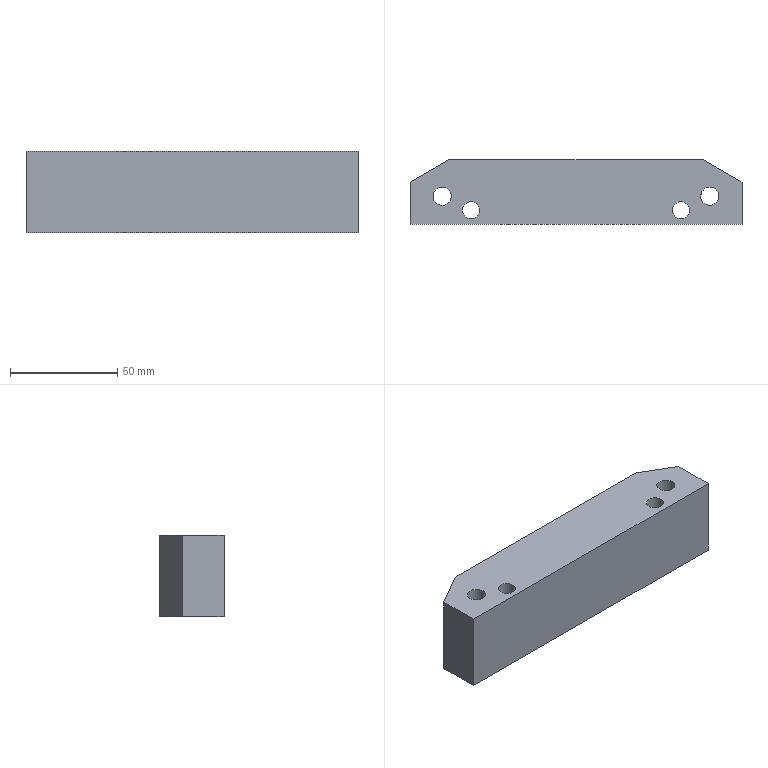Part | CATIA | 1 solid | 16 faces | box 155 x 30 x 38 mm | volume 161459 mm3 | plane 8 | cylinder 8 | commonest cylinder face diameters 8 x4 8.5 x4
STEP:
#1=CARTESIAN_POINT('',(77.5,-30.,38.));
#2=VERTEX_POINT('',#1);
#3=CARTESIAN_POINT('',(77.5,-30.,0.));
#4=VERTEX_POINT('',#3);
#5=CARTESIAN_POINT('',(77.5,-30.,19.));
#6=DIRECTION('',(0.,0.,-1.));
#7=VECTOR('',#6,1.);
#8=LINE('',#5,#7);
#9=EDGE_CURVE('',#2,#4,#8,.T.);
#10=ORIENTED_EDGE('',*,*,#9,.F.);
#11=CARTESIAN_POINT('',(-77.5,-30.,38.));
#12=VERTEX_POINT('',#11);
#13=CARTESIAN_POINT('',(0.,-30.,38.));
#14=DIRECTION('',(-1.,0.,0.));
#15=VECTOR('',#14,1.);
#16=LINE('',#13,#15);
#17=EDGE_CURVE('',#2,#12,#16,.T.);
#18=ORIENTED_EDGE('',*,*,#17,.T.);
#19=CARTESIAN_POINT('',(-77.5,-30.,0.));
#20=VERTEX_POINT('',#19);
#21=CARTESIAN_POINT('',(-77.5,-30.,19.));
#22=DIRECTION('',(0.,0.,-1.));
#23=VECTOR('',#22,1.);
#24=LINE('',#21,#23);
#25=EDGE_CURVE('',#12,#20,#24,.T.);
#26=ORIENTED_EDGE('',*,*,#25,.T.);
#27=CARTESIAN_POINT('',(0.,-30.,0.));
#28=DIRECTION('',(-1.,0.,0.));
#29=VECTOR('',#28,1.);
#30=LINE('',#27,#29);
#31=EDGE_CURVE('',#4,#20,#30,.T.);
#32=ORIENTED_EDGE('',*,*,#31,.F.);
#33=EDGE_LOOP('',(#10,#18,#26,#32));
#34=FACE_OUTER_BOUND('',#33,.T.);
#35=CARTESIAN_POINT('',(77.5,-30.,38.));
#36=DIRECTION('',(0.,-1.,0.));
#37=DIRECTION('',(-1.,0.,0.));
#38=AXIS2_PLACEMENT_3D('',#35,#36,#37);
#39=PLANE('',#38);
#40=ADVANCED_FACE('',(#34),#39,.T.);
#41=CARTESIAN_POINT('',(-77.5,-10.392,38.));
#42=VERTEX_POINT('',#41);
#43=CARTESIAN_POINT('',(-77.5,-10.392,0.));
#44=VERTEX_POINT('',#43);
#45=CARTESIAN_POINT('',(-77.5,-10.392,19.));
#46=DIRECTION('',(0.,0.,-1.));
#47=VECTOR('',#46,1.);
#48=LINE('',#45,#47);
#49=EDGE_CURVE('',#42,#44,#48,.T.);
#50=ORIENTED_EDGE('',*,*,#49,.T.);
#51=CARTESIAN_POINT('',(-77.5,-20.196,0.));
#52=DIRECTION('',(0.,-1.,0.));
#53=VECTOR('',#52,1.);
#54=LINE('',#51,#53);
#55=EDGE_CURVE('',#20,#44,#54,.F.);
#56=ORIENTED_EDGE('',*,*,#55,.F.);
#57=ORIENTED_EDGE('',*,*,#25,.F.);
#58=CARTESIAN_POINT('',(-77.5,-20.196,38.));
#59=DIRECTION('',(0.,-1.,0.));
#60=VECTOR('',#59,1.);
#61=LINE('',#58,#60);
#62=EDGE_CURVE('',#12,#42,#61,.F.);
#63=ORIENTED_EDGE('',*,*,#62,.T.);
#64=EDGE_LOOP('',(#50,#56,#57,#63));
#65=FACE_OUTER_BOUND('',#64,.T.);
#66=CARTESIAN_POINT('',(-77.5,0.,38.));
#67=DIRECTION('',(1.,0.,0.));
#68=DIRECTION('',(0.,-1.,0.));
#69=AXIS2_PLACEMENT_3D('',#66,#67,#68);
#70=PLANE('',#69);
#71=ADVANCED_FACE('',(#65),#70,.F.);
#72=CARTESIAN_POINT('',(-59.5,0.,0.));
#73=VERTEX_POINT('',#72);
#74=CARTESIAN_POINT('',(-68.5,-5.196,0.));
#75=DIRECTION('',(-0.866,-0.5,0.));
#76=VECTOR('',#75,1.);
#77=LINE('',#74,#76);
#78=EDGE_CURVE('',#73,#44,#77,.T.);
#79=ORIENTED_EDGE('',*,*,#78,.T.);
#80=ORIENTED_EDGE('',*,*,#49,.F.);
#81=CARTESIAN_POINT('',(-59.5,0.,38.));
#82=VERTEX_POINT('',#81);
#83=CARTESIAN_POINT('',(-68.5,-5.196,38.));
#84=DIRECTION('',(-0.866,-0.5,0.));
#85=VECTOR('',#84,1.);
#86=LINE('',#83,#85);
#87=EDGE_CURVE('',#42,#82,#86,.F.);
#88=ORIENTED_EDGE('',*,*,#87,.T.);
#89=CARTESIAN_POINT('',(-59.5,0.,19.));
#90=DIRECTION('',(0.,0.,-1.));
#91=VECTOR('',#90,1.);
#92=LINE('',#89,#91);
#93=EDGE_CURVE('',#82,#73,#92,.T.);
#94=ORIENTED_EDGE('',*,*,#93,.T.);
#95=EDGE_LOOP('',(#79,#80,#88,#94));
#96=FACE_OUTER_BOUND('',#95,.T.);
#97=CARTESIAN_POINT('',(-59.5,0.,45.6));
#98=DIRECTION('',(-0.5,0.866,0.));
#99=DIRECTION('',(0.,0.,-1.));
#100=AXIS2_PLACEMENT_3D('',#97,#98,#99);
#101=PLANE('',#100);
#102=ADVANCED_FACE('',(#96),#101,.T.);
#103=CARTESIAN_POINT('',(77.5,-10.392,38.));
#104=VERTEX_POINT('',#103);
#105=CARTESIAN_POINT('',(77.5,-10.392,0.));
#106=VERTEX_POINT('',#105);
#107=CARTESIAN_POINT('',(77.5,-10.392,19.));
#108=DIRECTION('',(0.,0.,1.));
#109=VECTOR('',#108,1.);
#110=LINE('',#107,#109);
#111=EDGE_CURVE('',#104,#106,#110,.F.);
#112=ORIENTED_EDGE('',*,*,#111,.F.);
#113=CARTESIAN_POINT('',(77.5,-20.196,38.));
#114=DIRECTION('',(0.,1.,0.));
#115=VECTOR('',#114,1.);
#116=LINE('',#113,#115);
#117=EDGE_CURVE('',#104,#2,#116,.F.);
#118=ORIENTED_EDGE('',*,*,#117,.T.);
#119=ORIENTED_EDGE('',*,*,#9,.T.);
#120=CARTESIAN_POINT('',(77.5,-20.196,0.));
#121=DIRECTION('',(0.,1.,0.));
#122=VECTOR('',#121,1.);
#123=LINE('',#120,#122);
#124=EDGE_CURVE('',#106,#4,#123,.F.);
#125=ORIENTED_EDGE('',*,*,#124,.F.);
#126=EDGE_LOOP('',(#112,#118,#119,#125));
#127=FACE_OUTER_BOUND('',#126,.T.);
#128=CARTESIAN_POINT('',(77.5,-30.,38.));
#129=DIRECTION('',(-1.,0.,0.));
#130=DIRECTION('',(0.,1.,0.));
#131=AXIS2_PLACEMENT_3D('',#128,#129,#130);
#132=PLANE('',#131);
#133=ADVANCED_FACE('',(#127),#132,.F.);
#134=CARTESIAN_POINT('',(59.5,0.,0.));
#135=VERTEX_POINT('',#134);
#136=CARTESIAN_POINT('',(0.,0.,0.));
#137=DIRECTION('',(1.,0.,0.));
#138=VECTOR('',#137,1.);
#139=LINE('',#136,#138);
#140=EDGE_CURVE('',#73,#135,#139,.T.);
#141=ORIENTED_EDGE('',*,*,#140,.F.);
#142=ORIENTED_EDGE('',*,*,#93,.F.);
#143=CARTESIAN_POINT('',(59.5,0.,38.));
#144=VERTEX_POINT('',#143);
#145=CARTESIAN_POINT('',(0.,0.,38.));
#146=DIRECTION('',(1.,0.,0.));
#147=VECTOR('',#146,1.);
#148=LINE('',#145,#147);
#149=EDGE_CURVE('',#82,#144,#148,.T.);
#150=ORIENTED_EDGE('',*,*,#149,.T.);
#151=CARTESIAN_POINT('',(59.5,0.,19.));
#152=DIRECTION('',(0.,0.,1.));
#153=VECTOR('',#152,1.);
#154=LINE('',#151,#153);
#155=EDGE_CURVE('',#144,#135,#154,.F.);
#156=ORIENTED_EDGE('',*,*,#155,.T.);
#157=EDGE_LOOP('',(#141,#142,#150,#156));
#158=FACE_OUTER_BOUND('',#157,.T.);
#159=CARTESIAN_POINT('',(-77.5,0.,38.));
#160=DIRECTION('',(0.,1.,0.));
#161=DIRECTION('',(1.,0.,0.));
#162=AXIS2_PLACEMENT_3D('',#159,#160,#161);
#163=PLANE('',#162);
#164=ADVANCED_FACE('',(#158),#163,.T.);
#165=CARTESIAN_POINT('',(68.5,-5.196,0.));
#166=DIRECTION('',(0.866,-0.5,0.));
#167=VECTOR('',#166,1.);
#168=LINE('',#165,#167);
#169=EDGE_CURVE('',#106,#135,#168,.F.);
#170=ORIENTED_EDGE('',*,*,#169,.T.);
#171=ORIENTED_EDGE('',*,*,#155,.F.);
#172=CARTESIAN_POINT('',(68.5,-5.196,38.));
#173=DIRECTION('',(0.866,-0.5,0.));
#174=VECTOR('',#173,1.);
#175=LINE('',#172,#174);
#176=EDGE_CURVE('',#144,#104,#175,.T.);
#177=ORIENTED_EDGE('',*,*,#176,.T.);
#178=ORIENTED_EDGE('',*,*,#111,.T.);
#179=EDGE_LOOP('',(#170,#171,#177,#178));
#180=FACE_OUTER_BOUND('',#179,.T.);
#181=CARTESIAN_POINT('',(59.5,0.,-7.6));
#182=DIRECTION('',(0.5,0.866,0.));
#183=DIRECTION('',(0.,0.,1.));
#184=AXIS2_PLACEMENT_3D('',#181,#182,#183);
#185=PLANE('',#184);
#186=ADVANCED_FACE('',(#180),#185,.T.);
#187=ORIENTED_EDGE('',*,*,#124,.T.);
#188=ORIENTED_EDGE('',*,*,#31,.T.);
#189=ORIENTED_EDGE('',*,*,#55,.T.);
#190=ORIENTED_EDGE('',*,*,#78,.F.);
#191=ORIENTED_EDGE('',*,*,#140,.T.);
#192=ORIENTED_EDGE('',*,*,#169,.F.);
#193=EDGE_LOOP('',(#187,#188,#189,#190,#191,#192));
#194=FACE_OUTER_BOUND('',#193,.T.);
#195=CARTESIAN_POINT('',(-66.23,-14.962,0.));
#196=VERTEX_POINT('',#195);
#197=CARTESIAN_POINT('',(-58.77,-19.038,0.));
#198=VERTEX_POINT('',#197);
#199=CARTESIAN_POINT('',(-62.5,-17.,0.));
#200=DIRECTION('',(0.,0.,-1.));
#201=AXIS2_PLACEMENT_3D('',#199,#200,$);
#202=CIRCLE('',#201,4.25);
#203=EDGE_CURVE('',#196,#198,#202,.T.);
#204=ORIENTED_EDGE('',*,*,#203,.F.);
#205=CARTESIAN_POINT('',(-62.5,-17.,0.));
#206=DIRECTION('',(0.,0.,-1.));
#207=AXIS2_PLACEMENT_3D('',#205,#206,$);
#208=CIRCLE('',#207,4.25);
#209=EDGE_CURVE('',#198,#196,#208,.T.);
#210=ORIENTED_EDGE('',*,*,#209,.F.);
#211=EDGE_LOOP('',(#204,#210));
#212=FACE_BOUND('',#211,.T.);
#213=CARTESIAN_POINT('',(58.77,-14.962,0.));
#214=VERTEX_POINT('',#213);
#215=CARTESIAN_POINT('',(66.23,-19.038,0.));
#216=VERTEX_POINT('',#215);
#217=CARTESIAN_POINT('',(62.5,-17.,0.));
#218=DIRECTION('',(0.,0.,-1.));
#219=AXIS2_PLACEMENT_3D('',#217,#218,$);
#220=CIRCLE('',#219,4.25);
#221=EDGE_CURVE('',#214,#216,#220,.T.);
#222=ORIENTED_EDGE('',*,*,#221,.F.);
#223=CARTESIAN_POINT('',(62.5,-17.,0.));
#224=DIRECTION('',(0.,0.,-1.));
#225=AXIS2_PLACEMENT_3D('',#223,#224,$);
#226=CIRCLE('',#225,4.25);
#227=EDGE_CURVE('',#216,#214,#226,.T.);
#228=ORIENTED_EDGE('',*,*,#227,.F.);
#229=EDGE_LOOP('',(#222,#228));
#230=FACE_BOUND('',#229,.T.);
#231=CARTESIAN_POINT('',(-52.51,-21.582,0.));
#232=VERTEX_POINT('',#231);
#233=CARTESIAN_POINT('',(-45.49,-25.418,0.));
#234=VERTEX_POINT('',#233);
#235=CARTESIAN_POINT('',(-49.,-23.5,0.));
#236=DIRECTION('',(0.,0.,-1.));
#237=AXIS2_PLACEMENT_3D('',#235,#236,$);
#238=CIRCLE('',#237,4.);
#239=EDGE_CURVE('',#232,#234,#238,.T.);
#240=ORIENTED_EDGE('',*,*,#239,.F.);
#241=CARTESIAN_POINT('',(-49.,-23.5,0.));
#242=DIRECTION('',(0.,0.,-1.));
#243=AXIS2_PLACEMENT_3D('',#241,#242,$);
#244=CIRCLE('',#243,4.);
#245=EDGE_CURVE('',#234,#232,#244,.T.);
#246=ORIENTED_EDGE('',*,*,#245,.F.);
#247=EDGE_LOOP('',(#240,#246));
#248=FACE_BOUND('',#247,.T.);
#249=CARTESIAN_POINT('',(45.49,-21.582,0.));
#250=VERTEX_POINT('',#249);
#251=CARTESIAN_POINT('',(52.51,-25.418,0.));
#252=VERTEX_POINT('',#251);
#253=CARTESIAN_POINT('',(49.,-23.5,0.));
#254=DIRECTION('',(0.,0.,-1.));
#255=AXIS2_PLACEMENT_3D('',#253,#254,$);
#256=CIRCLE('',#255,4.);
#257=EDGE_CURVE('',#250,#252,#256,.T.);
#258=ORIENTED_EDGE('',*,*,#257,.F.);
#259=CARTESIAN_POINT('',(49.,-23.5,0.));
#260=DIRECTION('',(0.,0.,-1.));
#261=AXIS2_PLACEMENT_3D('',#259,#260,$);
#262=CIRCLE('',#261,4.);
#263=EDGE_CURVE('',#252,#250,#262,.T.);
#264=ORIENTED_EDGE('',*,*,#263,.F.);
#265=EDGE_LOOP('',(#258,#264));
#266=FACE_BOUND('',#265,.T.);
#267=CARTESIAN_POINT('',(0.,0.,0.));
#268=DIRECTION('',(0.,0.,-1.));
#269=DIRECTION('',(1.,0.,0.));
#270=AXIS2_PLACEMENT_3D('',#267,#268,#269);
#271=PLANE('',#270);
#272=ADVANCED_FACE('',(#194,#212,#230,#248,#266),#271,.T.);
#273=ORIENTED_EDGE('',*,*,#176,.F.);
#274=ORIENTED_EDGE('',*,*,#149,.F.);
#275=ORIENTED_EDGE('',*,*,#87,.F.);
#276=ORIENTED_EDGE('',*,*,#62,.F.);
#277=ORIENTED_EDGE('',*,*,#17,.F.);
#278=ORIENTED_EDGE('',*,*,#117,.F.);
#279=EDGE_LOOP('',(#273,#274,#275,#276,#277,#278));
#280=FACE_OUTER_BOUND('',#279,.T.);
#281=CARTESIAN_POINT('',(-66.23,-14.962,38.));
#282=VERTEX_POINT('',#281);
#283=CARTESIAN_POINT('',(-58.77,-19.038,38.));
#284=VERTEX_POINT('',#283);
#285=CARTESIAN_POINT('',(-62.5,-17.,38.));
#286=DIRECTION('',(0.,0.,-1.));
#287=AXIS2_PLACEMENT_3D('',#285,#286,$);
#288=CIRCLE('',#287,4.25);
#289=EDGE_CURVE('',#282,#284,#288,.T.);
#290=ORIENTED_EDGE('',*,*,#289,.T.);
#291=CARTESIAN_POINT('',(-62.5,-17.,38.));
#292=DIRECTION('',(0.,0.,-1.));
#293=AXIS2_PLACEMENT_3D('',#291,#292,$);
#294=CIRCLE('',#293,4.25);
#295=EDGE_CURVE('',#284,#282,#294,.T.);
#296=ORIENTED_EDGE('',*,*,#295,.T.);
#297=EDGE_LOOP('',(#290,#296));
#298=FACE_BOUND('',#297,.T.);
#299=CARTESIAN_POINT('',(58.77,-14.962,38.));
#300=VERTEX_POINT('',#299);
#301=CARTESIAN_POINT('',(66.23,-19.038,38.));
#302=VERTEX_POINT('',#301);
#303=CARTESIAN_POINT('',(62.5,-17.,38.));
#304=DIRECTION('',(0.,0.,-1.));
#305=AXIS2_PLACEMENT_3D('',#303,#304,$);
#306=CIRCLE('',#305,4.25);
#307=EDGE_CURVE('',#300,#302,#306,.T.);
#308=ORIENTED_EDGE('',*,*,#307,.T.);
#309=CARTESIAN_POINT('',(62.5,-17.,38.));
#310=DIRECTION('',(0.,0.,-1.));
#311=AXIS2_PLACEMENT_3D('',#309,#310,$);
#312=CIRCLE('',#311,4.25);
#313=EDGE_CURVE('',#302,#300,#312,.T.);
#314=ORIENTED_EDGE('',*,*,#313,.T.);
#315=EDGE_LOOP('',(#308,#314));
#316=FACE_BOUND('',#315,.T.);
#317=CARTESIAN_POINT('',(-52.51,-21.582,38.));
#318=VERTEX_POINT('',#317);
#319=CARTESIAN_POINT('',(-45.49,-25.418,38.));
#320=VERTEX_POINT('',#319);
#321=CARTESIAN_POINT('',(-49.,-23.5,38.));
#322=DIRECTION('',(0.,0.,-1.));
#323=AXIS2_PLACEMENT_3D('',#321,#322,$);
#324=CIRCLE('',#323,4.);
#325=EDGE_CURVE('',#318,#320,#324,.T.);
#326=ORIENTED_EDGE('',*,*,#325,.T.);
#327=CARTESIAN_POINT('',(-49.,-23.5,38.));
#328=DIRECTION('',(0.,0.,-1.));
#329=AXIS2_PLACEMENT_3D('',#327,#328,$);
#330=CIRCLE('',#329,4.);
#331=EDGE_CURVE('',#320,#318,#330,.T.);
#332=ORIENTED_EDGE('',*,*,#331,.T.);
#333=EDGE_LOOP('',(#326,#332));
#334=FACE_BOUND('',#333,.T.);
#335=CARTESIAN_POINT('',(45.49,-21.582,38.));
#336=VERTEX_POINT('',#335);
#337=CARTESIAN_POINT('',(52.51,-25.418,38.));
#338=VERTEX_POINT('',#337);
#339=CARTESIAN_POINT('',(49.,-23.5,38.));
#340=DIRECTION('',(0.,0.,-1.));
#341=AXIS2_PLACEMENT_3D('',#339,#340,$);
#342=CIRCLE('',#341,4.);
#343=EDGE_CURVE('',#336,#338,#342,.T.);
#344=ORIENTED_EDGE('',*,*,#343,.T.);
#345=CARTESIAN_POINT('',(49.,-23.5,38.));
#346=DIRECTION('',(0.,0.,-1.));
#347=AXIS2_PLACEMENT_3D('',#345,#346,$);
#348=CIRCLE('',#347,4.);
#349=EDGE_CURVE('',#338,#336,#348,.T.);
#350=ORIENTED_EDGE('',*,*,#349,.T.);
#351=EDGE_LOOP('',(#344,#350));
#352=FACE_BOUND('',#351,.T.);
#353=CARTESIAN_POINT('',(0.,0.,38.));
#354=DIRECTION('',(0.,0.,-1.));
#355=DIRECTION('',(1.,0.,0.));
#356=AXIS2_PLACEMENT_3D('',#353,#354,#355);
#357=PLANE('',#356);
#358=ADVANCED_FACE('',(#280,#298,#316,#334,#352),#357,.F.);
#359=ORIENTED_EDGE('',*,*,#331,.F.);
#360=CARTESIAN_POINT('',(-45.49,-25.418,19.));
#361=DIRECTION('',(0.,0.,-1.));
#362=VECTOR('',#361,1.);
#363=LINE('',#360,#362);
#364=EDGE_CURVE('',#234,#320,#363,.F.);
#365=ORIENTED_EDGE('',*,*,#364,.F.);
#366=ORIENTED_EDGE('',*,*,#245,.T.);
#367=CARTESIAN_POINT('',(-52.51,-21.582,19.));
#368=DIRECTION('',(0.,0.,-1.));
#369=VECTOR('',#368,1.);
#370=LINE('',#367,#369);
#371=EDGE_CURVE('',#232,#318,#370,.F.);
#372=ORIENTED_EDGE('',*,*,#371,.T.);
#373=EDGE_LOOP('',(#359,#365,#366,#372));
#374=FACE_OUTER_BOUND('',#373,.T.);
#375=CARTESIAN_POINT('',(-49.,-23.5,37.9));
#376=DIRECTION('',(0.,0.,-1.));
#377=DIRECTION('',(0.8776,-0.4794,0.));
#378=AXIS2_PLACEMENT_3D('',#375,#376,#377);
#379=CYLINDRICAL_SURFACE('',#378,4.);
#380=ADVANCED_FACE('',(#374),#379,.F.);
#381=ORIENTED_EDGE('',*,*,#325,.F.);
#382=ORIENTED_EDGE('',*,*,#371,.F.);
#383=ORIENTED_EDGE('',*,*,#239,.T.);
#384=ORIENTED_EDGE('',*,*,#364,.T.);
#385=EDGE_LOOP('',(#381,#382,#383,#384));
#386=FACE_OUTER_BOUND('',#385,.T.);
#387=ADVANCED_FACE('',(#386),#379,.F.);
#388=ORIENTED_EDGE('',*,*,#313,.F.);
#389=CARTESIAN_POINT('',(66.23,-19.038,19.));
#390=DIRECTION('',(0.,0.,-1.));
#391=VECTOR('',#390,1.);
#392=LINE('',#389,#391);
#393=EDGE_CURVE('',#216,#302,#392,.F.);
#394=ORIENTED_EDGE('',*,*,#393,.F.);
#395=ORIENTED_EDGE('',*,*,#227,.T.);
#396=CARTESIAN_POINT('',(58.77,-14.962,19.));
#397=DIRECTION('',(0.,0.,-1.));
#398=VECTOR('',#397,1.);
#399=LINE('',#396,#398);
#400=EDGE_CURVE('',#214,#300,#399,.F.);
#401=ORIENTED_EDGE('',*,*,#400,.T.);
#402=EDGE_LOOP('',(#388,#394,#395,#401));
#403=FACE_OUTER_BOUND('',#402,.T.);
#404=CARTESIAN_POINT('',(62.5,-17.,37.9));
#405=DIRECTION('',(0.,0.,-1.));
#406=DIRECTION('',(0.8776,-0.4794,0.));
#407=AXIS2_PLACEMENT_3D('',#404,#405,#406);
#408=CYLINDRICAL_SURFACE('',#407,4.25);
#409=ADVANCED_FACE('',(#403),#408,.F.);
#410=ORIENTED_EDGE('',*,*,#307,.F.);
#411=ORIENTED_EDGE('',*,*,#400,.F.);
#412=ORIENTED_EDGE('',*,*,#221,.T.);
#413=ORIENTED_EDGE('',*,*,#393,.T.);
#414=EDGE_LOOP('',(#410,#411,#412,#413));
#415=FACE_OUTER_BOUND('',#414,.T.);
#416=ADVANCED_FACE('',(#415),#408,.F.);
#417=ORIENTED_EDGE('',*,*,#349,.F.);
#418=CARTESIAN_POINT('',(52.51,-25.418,19.));
#419=DIRECTION('',(0.,0.,-1.));
#420=VECTOR('',#419,1.);
#421=LINE('',#418,#420);
#422=EDGE_CURVE('',#252,#338,#421,.F.);
#423=ORIENTED_EDGE('',*,*,#422,.F.);
#424=ORIENTED_EDGE('',*,*,#263,.T.);
#425=CARTESIAN_POINT('',(45.49,-21.582,19.));
#426=DIRECTION('',(0.,0.,-1.));
#427=VECTOR('',#426,1.);
#428=LINE('',#425,#427);
#429=EDGE_CURVE('',#250,#336,#428,.F.);
#430=ORIENTED_EDGE('',*,*,#429,.T.);
#431=EDGE_LOOP('',(#417,#423,#424,#430));
#432=FACE_OUTER_BOUND('',#431,.T.);
#433=CARTESIAN_POINT('',(49.,-23.5,37.9));
#434=DIRECTION('',(0.,0.,-1.));
#435=DIRECTION('',(0.8776,-0.4794,0.));
#436=AXIS2_PLACEMENT_3D('',#433,#434,#435);
#437=CYLINDRICAL_SURFACE('',#436,4.);
#438=ADVANCED_FACE('',(#432),#437,.F.);
#439=ORIENTED_EDGE('',*,*,#343,.F.);
#440=ORIENTED_EDGE('',*,*,#429,.F.);
#441=ORIENTED_EDGE('',*,*,#257,.T.);
#442=ORIENTED_EDGE('',*,*,#422,.T.);
#443=EDGE_LOOP('',(#439,#440,#441,#442));
#444=FACE_OUTER_BOUND('',#443,.T.);
#445=ADVANCED_FACE('',(#444),#437,.F.);
#446=ORIENTED_EDGE('',*,*,#295,.F.);
#447=CARTESIAN_POINT('',(-58.77,-19.038,19.));
#448=DIRECTION('',(0.,0.,-1.));
#449=VECTOR('',#448,1.);
#450=LINE('',#447,#449);
#451=EDGE_CURVE('',#198,#284,#450,.F.);
#452=ORIENTED_EDGE('',*,*,#451,.F.);
#453=ORIENTED_EDGE('',*,*,#209,.T.);
#454=CARTESIAN_POINT('',(-66.23,-14.962,19.));
#455=DIRECTION('',(0.,0.,-1.));
#456=VECTOR('',#455,1.);
#457=LINE('',#454,#456);
#458=EDGE_CURVE('',#196,#282,#457,.F.);
#459=ORIENTED_EDGE('',*,*,#458,.T.);
#460=EDGE_LOOP('',(#446,#452,#453,#459));
#461=FACE_OUTER_BOUND('',#460,.T.);
#462=CARTESIAN_POINT('',(-62.5,-17.,37.9));
#463=DIRECTION('',(0.,0.,-1.));
#464=DIRECTION('',(0.8776,-0.4794,0.));
#465=AXIS2_PLACEMENT_3D('',#462,#463,#464);
#466=CYLINDRICAL_SURFACE('',#465,4.25);
#467=ADVANCED_FACE('',(#461),#466,.F.);
#468=ORIENTED_EDGE('',*,*,#289,.F.);
#469=ORIENTED_EDGE('',*,*,#458,.F.);
#470=ORIENTED_EDGE('',*,*,#203,.T.);
#471=ORIENTED_EDGE('',*,*,#451,.T.);
#472=EDGE_LOOP('',(#468,#469,#470,#471));
#473=FACE_OUTER_BOUND('',#472,.T.);
#474=ADVANCED_FACE('',(#473),#466,.F.);
#475=CLOSED_SHELL('',(#40,#71,#102,#133,#164,#186,#272,#358,#380,#387,#409,#416,#438,#445,#467,#474));
#476=MANIFOLD_SOLID_BREP('',#475);
#477=(LENGTH_UNIT()NAMED_UNIT(*)SI_UNIT(.MILLI.,.METRE.));
#478=UNCERTAINTY_MEASURE_WITH_UNIT(LENGTH_MEASURE(0.005),#477,'','');
#479=(NAMED_UNIT(*)PLANE_ANGLE_UNIT()SI_UNIT($,.RADIAN.));
#480=(NAMED_UNIT(*)SI_UNIT($,.STERADIAN.)SOLID_ANGLE_UNIT());
#481=(GEOMETRIC_REPRESENTATION_CONTEXT(3)GLOBAL_UNCERTAINTY_ASSIGNED_CONTEXT((#478))GLOBAL_UNIT_ASSIGNED_CONTEXT((#477,#479,#480))REPRESENTATION_CONTEXT('',''));
#482=ADVANCED_BREP_SHAPE_REPRESENTATION('',(#476),#481);